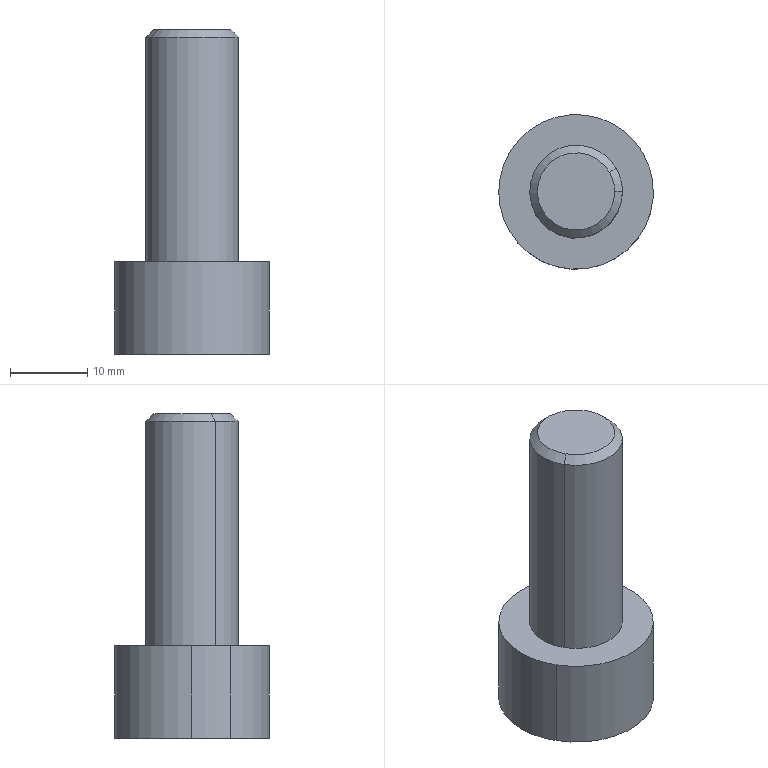Part | SolidWorks | features BaseBody 1 | 1 solid | 19 faces | box 20 x 20 x 42 mm | volume 6635 mm3 | plane 10 | cylinder 6 | cone 3 | commonest cylinder face diameters 12 x3 20 x3
STEP:
#1=CARTESIAN_POINT('',(127.379,873.749,686.107));
#2=VERTEX_POINT('',#1);
#3=CARTESIAN_POINT('',(128.245,874.249,685.107));
#4=VERTEX_POINT('',#3);
#5=CARTESIAN_POINT('',(127.379,873.749,686.107));
#6=DIRECTION('',(0.6124,0.3536,-0.7071));
#7=VECTOR('',#6,1000.);
#8=LINE('',#5,#7);
#9=EDGE_CURVE('',#2,#4,#8,.T.);
#10=ORIENTED_EDGE('',*,*,#9,.T.);
#11=CARTESIAN_POINT('',(117.853,868.249,685.107));
#12=VERTEX_POINT('',#11);
#13=CARTESIAN_POINT('',(123.049,871.249,685.107));
#14=DIRECTION('',(0.,0.,1.));
#15=DIRECTION('',(0.866,0.5,0.));
#16=AXIS2_PLACEMENT_3D('',#13,#14,#15);
#17=CIRCLE('',#16,6.);
#18=EDGE_CURVE('',#4,#12,#17,.T.);
#19=ORIENTED_EDGE('',*,*,#18,.T.);
#20=CARTESIAN_POINT('',(118.719,868.749,686.107));
#21=VERTEX_POINT('',#20);
#22=CARTESIAN_POINT('',(118.719,868.749,686.107));
#23=DIRECTION('',(-0.6124,-0.3536,-0.7071));
#24=VECTOR('',#23,1000.);
#25=LINE('',#22,#24);
#26=EDGE_CURVE('',#21,#12,#25,.T.);
#27=ORIENTED_EDGE('',*,*,#26,.F.);
#28=CARTESIAN_POINT('',(123.049,871.249,686.107));
#29=DIRECTION('',(0.,0.,-1.));
#30=DIRECTION('',(0.866,0.5,0.));
#31=AXIS2_PLACEMENT_3D('',#28,#29,#30);
#32=CIRCLE('',#31,5.);
#33=EDGE_CURVE('',#21,#2,#32,.T.);
#34=ORIENTED_EDGE('',*,*,#33,.T.);
#35=EDGE_LOOP('',(#10,#19,#27,#34));
#36=FACE_OUTER_BOUND('',#35,.T.);
#37=CARTESIAN_POINT('',(123.049,871.249,686.107));
#38=DIRECTION('',(0.,0.,-1.));
#39=DIRECTION('',(1.,0.,0.));
#40=AXIS2_PLACEMENT_3D('',#37,#38,#39);
#41=CONICAL_SURFACE('',#40,5.,0.7854);
#42=ADVANCED_FACE('',(#36),#41,.T.);
#43=ORIENTED_EDGE('',*,*,#33,.F.);
#44=CARTESIAN_POINT('',(128.049,871.249,686.107));
#45=VERTEX_POINT('',#44);
#46=CARTESIAN_POINT('',(123.049,871.249,686.107));
#47=DIRECTION('',(0.,0.,-1.));
#48=DIRECTION('',(0.866,0.5,0.));
#49=AXIS2_PLACEMENT_3D('',#46,#47,#48);
#50=CIRCLE('',#49,5.);
#51=EDGE_CURVE('',#45,#21,#50,.T.);
#52=ORIENTED_EDGE('',*,*,#51,.F.);
#53=CARTESIAN_POINT('',(123.049,871.249,686.107));
#54=DIRECTION('',(0.,0.,-1.));
#55=DIRECTION('',(0.866,0.5,0.));
#56=AXIS2_PLACEMENT_3D('',#53,#54,#55);
#57=CIRCLE('',#56,5.);
#58=EDGE_CURVE('',#2,#45,#57,.T.);
#59=ORIENTED_EDGE('',*,*,#58,.F.);
#60=EDGE_LOOP('',(#43,#52,#59));
#61=FACE_OUTER_BOUND('',#60,.T.);
#62=CARTESIAN_POINT('',(123.049,871.249,686.107));
#63=DIRECTION('',(0.,0.,1.));
#64=DIRECTION('',(1.,0.,0.));
#65=AXIS2_PLACEMENT_3D('',#62,#63,#64);
#66=PLANE('',#65);
#67=ADVANCED_FACE('',(#61),#66,.T.);
#68=CARTESIAN_POINT('',(128.245,874.249,656.107));
#69=VERTEX_POINT('',#68);
#70=CARTESIAN_POINT('',(128.245,874.249,686.107));
#71=DIRECTION('',(0.,0.,-1.));
#72=VECTOR('',#71,1000.);
#73=LINE('',#70,#72);
#74=EDGE_CURVE('',#4,#69,#73,.T.);
#75=ORIENTED_EDGE('',*,*,#74,.T.);
#76=CARTESIAN_POINT('',(117.853,868.249,656.107));
#77=VERTEX_POINT('',#76);
#78=CARTESIAN_POINT('',(123.049,871.249,656.107));
#79=DIRECTION('',(0.,0.,-1.));
#80=DIRECTION('',(-0.866,-0.5,0.));
#81=AXIS2_PLACEMENT_3D('',#78,#79,#80);
#82=CIRCLE('',#81,6.);
#83=EDGE_CURVE('',#77,#69,#82,.T.);
#84=ORIENTED_EDGE('',*,*,#83,.F.);
#85=CARTESIAN_POINT('',(117.853,868.249,686.107));
#86=DIRECTION('',(0.,0.,-1.));
#87=VECTOR('',#86,1000.);
#88=LINE('',#85,#87);
#89=EDGE_CURVE('',#12,#77,#88,.T.);
#90=ORIENTED_EDGE('',*,*,#89,.F.);
#91=ORIENTED_EDGE('',*,*,#18,.F.);
#92=EDGE_LOOP('',(#75,#84,#90,#91));
#93=FACE_OUTER_BOUND('',#92,.T.);
#94=CARTESIAN_POINT('',(123.049,871.249,686.107));
#95=DIRECTION('',(0.,0.,-1.));
#96=DIRECTION('',(1.,0.,0.));
#97=AXIS2_PLACEMENT_3D('',#94,#95,#96);
#98=CYLINDRICAL_SURFACE('',#97,6.);
#99=ADVANCED_FACE('',(#93),#98,.T.);
#100=CARTESIAN_POINT('',(121.262,876.683,650.107));
#101=VERTEX_POINT('',#100);
#102=CARTESIAN_POINT('',(117.449,872.418,650.107));
#103=VERTEX_POINT('',#102);
#104=CARTESIAN_POINT('',(121.262,876.683,650.107));
#105=DIRECTION('',(-0.6665,-0.7455,0.));
#106=VECTOR('',#105,1000.);
#107=LINE('',#104,#106);
#108=EDGE_CURVE('',#101,#103,#107,.T.);
#109=ORIENTED_EDGE('',*,*,#108,.F.);
#110=CARTESIAN_POINT('',(126.861,875.513,650.107));
#111=VERTEX_POINT('',#110);
#112=CARTESIAN_POINT('',(126.861,875.513,650.107));
#113=DIRECTION('',(-0.9789,0.2044,0.));
#114=VECTOR('',#113,1000.);
#115=LINE('',#112,#114);
#116=EDGE_CURVE('',#111,#101,#115,.T.);
#117=ORIENTED_EDGE('',*,*,#116,.F.);
#118=CARTESIAN_POINT('',(128.648,870.08,650.107));
#119=VERTEX_POINT('',#118);
#120=CARTESIAN_POINT('',(128.648,870.08,650.107));
#121=DIRECTION('',(-0.3124,0.9499,0.));
#122=VECTOR('',#121,1000.);
#123=LINE('',#120,#122);
#124=EDGE_CURVE('',#119,#111,#123,.T.);
#125=ORIENTED_EDGE('',*,*,#124,.F.);
#126=CARTESIAN_POINT('',(124.836,865.815,650.107));
#127=VERTEX_POINT('',#126);
#128=CARTESIAN_POINT('',(124.836,865.815,650.107));
#129=DIRECTION('',(0.6665,0.7455,0.));
#130=VECTOR('',#129,1000.);
#131=LINE('',#128,#130);
#132=EDGE_CURVE('',#127,#119,#131,.T.);
#133=ORIENTED_EDGE('',*,*,#132,.F.);
#134=CARTESIAN_POINT('',(119.237,866.984,650.107));
#135=VERTEX_POINT('',#134);
#136=CARTESIAN_POINT('',(119.237,866.984,650.107));
#137=DIRECTION('',(0.9789,-0.2044,0.));
#138=VECTOR('',#137,1000.);
#139=LINE('',#136,#138);
#140=EDGE_CURVE('',#135,#127,#139,.T.);
#141=ORIENTED_EDGE('',*,*,#140,.F.);
#142=CARTESIAN_POINT('',(117.449,872.418,650.107));
#143=DIRECTION('',(0.3124,-0.9499,0.));
#144=VECTOR('',#143,1000.);
#145=LINE('',#142,#144);
#146=EDGE_CURVE('',#103,#135,#145,.T.);
#147=ORIENTED_EDGE('',*,*,#146,.F.);
#148=EDGE_LOOP('',(#109,#117,#125,#133,#141,#147));
#149=FACE_OUTER_BOUND('',#148,.T.);
#150=CARTESIAN_POINT('',(117.449,872.418,650.107));
#151=DIRECTION('',(0.,0.,-1.));
#152=DIRECTION('',(0.,-1.,0.));
#153=AXIS2_PLACEMENT_3D('',#150,#151,#152);
#154=PLANE('',#153);
#155=ADVANCED_FACE('',(#149),#154,.T.);
#156=CARTESIAN_POINT('',(117.449,872.418,644.107));
#157=VERTEX_POINT('',#156);
#158=CARTESIAN_POINT('',(119.237,866.984,644.107));
#159=VERTEX_POINT('',#158);
#160=CARTESIAN_POINT('',(117.449,872.418,644.107));
#161=DIRECTION('',(0.3124,-0.9499,0.));
#162=VECTOR('',#161,1000.);
#163=LINE('',#160,#162);
#164=EDGE_CURVE('',#157,#159,#163,.T.);
#165=ORIENTED_EDGE('',*,*,#164,.F.);
#166=CARTESIAN_POINT('',(117.449,872.418,650.107));
#167=DIRECTION('',(0.,0.,-1.));
#168=VECTOR('',#167,1000.);
#169=LINE('',#166,#168);
#170=EDGE_CURVE('',#103,#157,#169,.T.);
#171=ORIENTED_EDGE('',*,*,#170,.F.);
#172=ORIENTED_EDGE('',*,*,#146,.T.);
#173=CARTESIAN_POINT('',(119.237,866.984,650.107));
#174=DIRECTION('',(0.,0.,-1.));
#175=VECTOR('',#174,1000.);
#176=LINE('',#173,#175);
#177=EDGE_CURVE('',#135,#159,#176,.T.);
#178=ORIENTED_EDGE('',*,*,#177,.T.);
#179=EDGE_LOOP('',(#165,#171,#172,#178));
#180=FACE_OUTER_BOUND('',#179,.T.);
#181=CARTESIAN_POINT('',(117.449,872.418,650.107));
#182=DIRECTION('',(-0.9499,-0.3124,0.));
#183=DIRECTION('',(-0.3124,0.9499,0.));
#184=AXIS2_PLACEMENT_3D('',#181,#182,#183);
#185=PLANE('',#184);
#186=ADVANCED_FACE('',(#180),#185,.F.);
#187=CARTESIAN_POINT('',(124.836,865.815,644.107));
#188=VERTEX_POINT('',#187);
#189=CARTESIAN_POINT('',(119.237,866.984,644.107));
#190=DIRECTION('',(0.9789,-0.2044,0.));
#191=VECTOR('',#190,1000.);
#192=LINE('',#189,#191);
#193=EDGE_CURVE('',#159,#188,#192,.T.);
#194=ORIENTED_EDGE('',*,*,#193,.F.);
#195=ORIENTED_EDGE('',*,*,#177,.F.);
#196=ORIENTED_EDGE('',*,*,#140,.T.);
#197=CARTESIAN_POINT('',(124.836,865.815,650.107));
#198=DIRECTION('',(0.,0.,-1.));
#199=VECTOR('',#198,1000.);
#200=LINE('',#197,#199);
#201=EDGE_CURVE('',#127,#188,#200,.T.);
#202=ORIENTED_EDGE('',*,*,#201,.T.);
#203=EDGE_LOOP('',(#194,#195,#196,#202));
#204=FACE_OUTER_BOUND('',#203,.T.);
#205=CARTESIAN_POINT('',(119.237,866.984,650.107));
#206=DIRECTION('',(-0.2044,-0.9789,0.));
#207=DIRECTION('',(-0.9789,0.2044,0.));
#208=AXIS2_PLACEMENT_3D('',#205,#206,#207);
#209=PLANE('',#208);
#210=ADVANCED_FACE('',(#204),#209,.F.);
#211=CARTESIAN_POINT('',(128.648,870.08,644.107));
#212=VERTEX_POINT('',#211);
#213=CARTESIAN_POINT('',(124.836,865.815,644.107));
#214=DIRECTION('',(0.6665,0.7455,0.));
#215=VECTOR('',#214,1000.);
#216=LINE('',#213,#215);
#217=EDGE_CURVE('',#188,#212,#216,.T.);
#218=ORIENTED_EDGE('',*,*,#217,.F.);
#219=ORIENTED_EDGE('',*,*,#201,.F.);
#220=ORIENTED_EDGE('',*,*,#132,.T.);
#221=CARTESIAN_POINT('',(128.648,870.08,650.107));
#222=DIRECTION('',(0.,0.,-1.));
#223=VECTOR('',#222,1000.);
#224=LINE('',#221,#223);
#225=EDGE_CURVE('',#119,#212,#224,.T.);
#226=ORIENTED_EDGE('',*,*,#225,.T.);
#227=EDGE_LOOP('',(#218,#219,#220,#226));
#228=FACE_OUTER_BOUND('',#227,.T.);
#229=CARTESIAN_POINT('',(124.836,865.815,650.107));
#230=DIRECTION('',(0.7455,-0.6665,0.));
#231=DIRECTION('',(0.,0.,-1.));
#232=AXIS2_PLACEMENT_3D('',#229,#230,#231);
#233=PLANE('',#232);
#234=ADVANCED_FACE('',(#228),#233,.F.);
#235=CARTESIAN_POINT('',(126.861,875.513,644.107));
#236=VERTEX_POINT('',#235);
#237=CARTESIAN_POINT('',(128.648,870.08,644.107));
#238=DIRECTION('',(-0.3124,0.9499,0.));
#239=VECTOR('',#238,1000.);
#240=LINE('',#237,#239);
#241=EDGE_CURVE('',#212,#236,#240,.T.);
#242=ORIENTED_EDGE('',*,*,#241,.F.);
#243=ORIENTED_EDGE('',*,*,#225,.F.);
#244=ORIENTED_EDGE('',*,*,#124,.T.);
#245=CARTESIAN_POINT('',(126.861,875.513,650.107));
#246=DIRECTION('',(0.,0.,-1.));
#247=VECTOR('',#246,1000.);
#248=LINE('',#245,#247);
#249=EDGE_CURVE('',#111,#236,#248,.T.);
#250=ORIENTED_EDGE('',*,*,#249,.T.);
#251=EDGE_LOOP('',(#242,#243,#244,#250));
#252=FACE_OUTER_BOUND('',#251,.T.);
#253=CARTESIAN_POINT('',(128.648,870.08,650.107));
#254=DIRECTION('',(0.9499,0.3124,0.));
#255=DIRECTION('',(0.,0.,-1.));
#256=AXIS2_PLACEMENT_3D('',#253,#254,#255);
#257=PLANE('',#256);
#258=ADVANCED_FACE('',(#252),#257,.F.);
#259=CARTESIAN_POINT('',(121.262,876.683,644.107));
#260=VERTEX_POINT('',#259);
#261=CARTESIAN_POINT('',(126.861,875.513,644.107));
#262=DIRECTION('',(-0.9789,0.2044,0.));
#263=VECTOR('',#262,1000.);
#264=LINE('',#261,#263);
#265=EDGE_CURVE('',#236,#260,#264,.T.);
#266=ORIENTED_EDGE('',*,*,#265,.F.);
#267=ORIENTED_EDGE('',*,*,#249,.F.);
#268=ORIENTED_EDGE('',*,*,#116,.T.);
#269=CARTESIAN_POINT('',(121.262,876.683,650.107));
#270=DIRECTION('',(0.,0.,-1.));
#271=VECTOR('',#270,1000.);
#272=LINE('',#269,#271);
#273=EDGE_CURVE('',#101,#260,#272,.T.);
#274=ORIENTED_EDGE('',*,*,#273,.T.);
#275=EDGE_LOOP('',(#266,#267,#268,#274));
#276=FACE_OUTER_BOUND('',#275,.T.);
#277=CARTESIAN_POINT('',(126.861,875.513,650.107));
#278=DIRECTION('',(0.2044,0.9789,0.));
#279=DIRECTION('',(0.,0.,-1.));
#280=AXIS2_PLACEMENT_3D('',#277,#278,#279);
#281=PLANE('',#280);
#282=ADVANCED_FACE('',(#276),#281,.F.);
#283=CARTESIAN_POINT('',(121.262,876.683,644.107));
#284=DIRECTION('',(-0.6665,-0.7455,0.));
#285=VECTOR('',#284,1000.);
#286=LINE('',#283,#285);
#287=EDGE_CURVE('',#260,#157,#286,.T.);
#288=ORIENTED_EDGE('',*,*,#287,.F.);
#289=ORIENTED_EDGE('',*,*,#273,.F.);
#290=ORIENTED_EDGE('',*,*,#108,.T.);
#291=ORIENTED_EDGE('',*,*,#170,.T.);
#292=EDGE_LOOP('',(#288,#289,#290,#291));
#293=FACE_OUTER_BOUND('',#292,.T.);
#294=CARTESIAN_POINT('',(121.262,876.683,650.107));
#295=DIRECTION('',(-0.7455,0.6665,0.));
#296=DIRECTION('',(0.,0.,1.));
#297=AXIS2_PLACEMENT_3D('',#294,#295,#296);
#298=PLANE('',#297);
#299=ADVANCED_FACE('',(#293),#298,.F.);
#300=ORIENTED_EDGE('',*,*,#287,.T.);
#301=ORIENTED_EDGE('',*,*,#164,.T.);
#302=ORIENTED_EDGE('',*,*,#193,.T.);
#303=ORIENTED_EDGE('',*,*,#217,.T.);
#304=ORIENTED_EDGE('',*,*,#241,.T.);
#305=ORIENTED_EDGE('',*,*,#265,.T.);
#306=EDGE_LOOP('',(#300,#301,#302,#303,#304,#305));
#307=FACE_BOUND('',#306,.T.);
#308=CARTESIAN_POINT('',(131.709,876.249,644.107));
#309=VERTEX_POINT('',#308);
#310=CARTESIAN_POINT('',(113.049,871.249,644.107));
#311=VERTEX_POINT('',#310);
#312=CARTESIAN_POINT('',(123.049,871.249,644.107));
#313=DIRECTION('',(0.,0.,1.));
#314=DIRECTION('',(-0.866,-0.5,0.));
#315=AXIS2_PLACEMENT_3D('',#312,#313,#314);
#316=CIRCLE('',#315,10.);
#317=EDGE_CURVE('',#309,#311,#316,.T.);
#318=ORIENTED_EDGE('',*,*,#317,.F.);
#319=CARTESIAN_POINT('',(114.388,866.249,644.107));
#320=VERTEX_POINT('',#319);
#321=CARTESIAN_POINT('',(123.049,871.249,644.107));
#322=DIRECTION('',(0.,0.,1.));
#323=DIRECTION('',(-0.866,-0.5,0.));
#324=AXIS2_PLACEMENT_3D('',#321,#322,#323);
#325=CIRCLE('',#324,10.);
#326=EDGE_CURVE('',#320,#309,#325,.T.);
#327=ORIENTED_EDGE('',*,*,#326,.F.);
#328=CARTESIAN_POINT('',(123.049,871.249,644.107));
#329=DIRECTION('',(0.,0.,1.));
#330=DIRECTION('',(-0.866,-0.5,0.));
#331=AXIS2_PLACEMENT_3D('',#328,#329,#330);
#332=CIRCLE('',#331,10.);
#333=EDGE_CURVE('',#311,#320,#332,.T.);
#334=ORIENTED_EDGE('',*,*,#333,.F.);
#335=EDGE_LOOP('',(#318,#327,#334));
#336=FACE_OUTER_BOUND('',#335,.T.);
#337=CARTESIAN_POINT('',(123.049,871.249,644.107));
#338=DIRECTION('',(0.,0.,-1.));
#339=DIRECTION('',(0.,-1.,0.));
#340=AXIS2_PLACEMENT_3D('',#337,#338,#339);
#341=PLANE('',#340);
#342=ADVANCED_FACE('',(#307,#336),#341,.T.);
#343=CARTESIAN_POINT('',(113.049,871.249,656.107));
#344=VERTEX_POINT('',#343);
#345=CARTESIAN_POINT('',(113.049,871.249,644.107));
#346=DIRECTION('',(0.,0.,1.));
#347=VECTOR('',#346,1000.);
#348=LINE('',#345,#347);
#349=EDGE_CURVE('',#311,#344,#348,.T.);
#350=ORIENTED_EDGE('',*,*,#349,.F.);
#351=ORIENTED_EDGE('',*,*,#333,.T.);
#352=CARTESIAN_POINT('',(114.388,866.249,656.107));
#353=VERTEX_POINT('',#352);
#354=CARTESIAN_POINT('',(114.388,866.249,644.107));
#355=DIRECTION('',(0.,0.,1.));
#356=VECTOR('',#355,1000.);
#357=LINE('',#354,#356);
#358=EDGE_CURVE('',#320,#353,#357,.T.);
#359=ORIENTED_EDGE('',*,*,#358,.T.);
#360=CARTESIAN_POINT('',(123.049,871.249,656.107));
#361=DIRECTION('',(0.,0.,1.));
#362=DIRECTION('',(-0.866,-0.5,0.));
#363=AXIS2_PLACEMENT_3D('',#360,#361,#362);
#364=CIRCLE('',#363,10.);
#365=EDGE_CURVE('',#344,#353,#364,.T.);
#366=ORIENTED_EDGE('',*,*,#365,.F.);
#367=EDGE_LOOP('',(#350,#351,#359,#366));
#368=FACE_OUTER_BOUND('',#367,.T.);
#369=CARTESIAN_POINT('',(123.049,871.249,644.107));
#370=DIRECTION('',(0.,0.,1.));
#371=DIRECTION('',(-1.,0.,0.));
#372=AXIS2_PLACEMENT_3D('',#369,#370,#371);
#373=CYLINDRICAL_SURFACE('',#372,10.);
#374=ADVANCED_FACE('',(#368),#373,.T.);
#375=ORIENTED_EDGE('',*,*,#83,.T.);
#376=CARTESIAN_POINT('',(129.049,871.249,656.107));
#377=VERTEX_POINT('',#376);
#378=CARTESIAN_POINT('',(123.049,871.249,656.107));
#379=DIRECTION('',(0.,0.,-1.));
#380=DIRECTION('',(-0.866,-0.5,0.));
#381=AXIS2_PLACEMENT_3D('',#378,#379,#380);
#382=CIRCLE('',#381,6.);
#383=EDGE_CURVE('',#69,#377,#382,.T.);
#384=ORIENTED_EDGE('',*,*,#383,.T.);
#385=CARTESIAN_POINT('',(123.049,871.249,656.107));
#386=DIRECTION('',(0.,0.,-1.));
#387=DIRECTION('',(-0.866,-0.5,0.));
#388=AXIS2_PLACEMENT_3D('',#385,#386,#387);
#389=CIRCLE('',#388,6.);
#390=EDGE_CURVE('',#377,#77,#389,.T.);
#391=ORIENTED_EDGE('',*,*,#390,.T.);
#392=EDGE_LOOP('',(#375,#384,#391));
#393=FACE_BOUND('',#392,.T.);
#394=CARTESIAN_POINT('',(131.709,876.249,656.107));
#395=VERTEX_POINT('',#394);
#396=CARTESIAN_POINT('',(123.049,871.249,656.107));
#397=DIRECTION('',(0.,0.,1.));
#398=DIRECTION('',(-0.866,-0.5,0.));
#399=AXIS2_PLACEMENT_3D('',#396,#397,#398);
#400=CIRCLE('',#399,10.);
#401=EDGE_CURVE('',#395,#344,#400,.T.);
#402=ORIENTED_EDGE('',*,*,#401,.T.);
#403=ORIENTED_EDGE('',*,*,#365,.T.);
#404=CARTESIAN_POINT('',(123.049,871.249,656.107));
#405=DIRECTION('',(0.,0.,1.));
#406=DIRECTION('',(-0.866,-0.5,0.));
#407=AXIS2_PLACEMENT_3D('',#404,#405,#406);
#408=CIRCLE('',#407,10.);
#409=EDGE_CURVE('',#353,#395,#408,.T.);
#410=ORIENTED_EDGE('',*,*,#409,.T.);
#411=EDGE_LOOP('',(#402,#403,#410));
#412=FACE_OUTER_BOUND('',#411,.T.);
#413=CARTESIAN_POINT('',(123.049,871.249,656.107));
#414=DIRECTION('',(0.,0.,-1.));
#415=DIRECTION('',(0.,-1.,0.));
#416=AXIS2_PLACEMENT_3D('',#413,#414,#415);
#417=PLANE('',#416);
#418=ADVANCED_FACE('',(#393,#412),#417,.F.);
#419=ORIENTED_EDGE('',*,*,#326,.T.);
#420=CARTESIAN_POINT('',(131.709,876.249,644.107));
#421=DIRECTION('',(0.,0.,1.));
#422=VECTOR('',#421,1000.);
#423=LINE('',#420,#422);
#424=EDGE_CURVE('',#309,#395,#423,.T.);
#425=ORIENTED_EDGE('',*,*,#424,.T.);
#426=ORIENTED_EDGE('',*,*,#409,.F.);
#427=ORIENTED_EDGE('',*,*,#358,.F.);
#428=EDGE_LOOP('',(#419,#425,#426,#427));
#429=FACE_OUTER_BOUND('',#428,.T.);
#430=CARTESIAN_POINT('',(123.049,871.249,644.107));
#431=DIRECTION('',(0.,0.,1.));
#432=DIRECTION('',(-1.,0.,0.));
#433=AXIS2_PLACEMENT_3D('',#430,#431,#432);
#434=CYLINDRICAL_SURFACE('',#433,10.);
#435=ADVANCED_FACE('',(#429),#434,.T.);
#436=CARTESIAN_POINT('',(129.049,871.249,685.107));
#437=VERTEX_POINT('',#436);
#438=CARTESIAN_POINT('',(129.049,871.249,686.107));
#439=DIRECTION('',(0.,0.,-1.));
#440=VECTOR('',#439,1000.);
#441=LINE('',#438,#440);
#442=EDGE_CURVE('',#437,#377,#441,.T.);
#443=ORIENTED_EDGE('',*,*,#442,.F.);
#444=CARTESIAN_POINT('',(123.049,871.249,685.107));
#445=DIRECTION('',(0.,0.,1.));
#446=DIRECTION('',(0.866,0.5,0.));
#447=AXIS2_PLACEMENT_3D('',#444,#445,#446);
#448=CIRCLE('',#447,6.);
#449=EDGE_CURVE('',#12,#437,#448,.T.);
#450=ORIENTED_EDGE('',*,*,#449,.F.);
#451=ORIENTED_EDGE('',*,*,#89,.T.);
#452=ORIENTED_EDGE('',*,*,#390,.F.);
#453=EDGE_LOOP('',(#443,#450,#451,#452));
#454=FACE_OUTER_BOUND('',#453,.T.);
#455=CARTESIAN_POINT('',(123.049,871.249,686.107));
#456=DIRECTION('',(0.,0.,-1.));
#457=DIRECTION('',(1.,0.,0.));
#458=AXIS2_PLACEMENT_3D('',#455,#456,#457);
#459=CYLINDRICAL_SURFACE('',#458,6.);
#460=ADVANCED_FACE('',(#454),#459,.T.);
#461=CARTESIAN_POINT('',(128.049,871.249,686.107));
#462=DIRECTION('',(0.7071,0.,-0.7071));
#463=VECTOR('',#462,1000.);
#464=LINE('',#461,#463);
#465=EDGE_CURVE('',#45,#437,#464,.T.);
#466=ORIENTED_EDGE('',*,*,#465,.F.);
#467=ORIENTED_EDGE('',*,*,#51,.T.);
#468=ORIENTED_EDGE('',*,*,#26,.T.);
#469=ORIENTED_EDGE('',*,*,#449,.T.);
#470=EDGE_LOOP('',(#466,#467,#468,#469));
#471=FACE_OUTER_BOUND('',#470,.T.);
#472=CARTESIAN_POINT('',(123.049,871.249,686.107));
#473=DIRECTION('',(0.,0.,-1.));
#474=DIRECTION('',(1.,0.,0.));
#475=AXIS2_PLACEMENT_3D('',#472,#473,#474);
#476=CONICAL_SURFACE('',#475,5.,0.7854);
#477=ADVANCED_FACE('',(#471),#476,.T.);
#478=ORIENTED_EDGE('',*,*,#58,.T.);
#479=ORIENTED_EDGE('',*,*,#465,.T.);
#480=CARTESIAN_POINT('',(123.049,871.249,685.107));
#481=DIRECTION('',(0.,0.,1.));
#482=DIRECTION('',(0.866,0.5,0.));
#483=AXIS2_PLACEMENT_3D('',#480,#481,#482);
#484=CIRCLE('',#483,6.);
#485=EDGE_CURVE('',#437,#4,#484,.T.);
#486=ORIENTED_EDGE('',*,*,#485,.T.);
#487=ORIENTED_EDGE('',*,*,#9,.F.);
#488=EDGE_LOOP('',(#478,#479,#486,#487));
#489=FACE_OUTER_BOUND('',#488,.T.);
#490=CARTESIAN_POINT('',(123.049,871.249,686.107));
#491=DIRECTION('',(0.,0.,-1.));
#492=DIRECTION('',(1.,0.,0.));
#493=AXIS2_PLACEMENT_3D('',#490,#491,#492);
#494=CONICAL_SURFACE('',#493,5.,0.7854);
#495=ADVANCED_FACE('',(#489),#494,.T.);
#496=ORIENTED_EDGE('',*,*,#485,.F.);
#497=ORIENTED_EDGE('',*,*,#442,.T.);
#498=ORIENTED_EDGE('',*,*,#383,.F.);
#499=ORIENTED_EDGE('',*,*,#74,.F.);
#500=EDGE_LOOP('',(#496,#497,#498,#499));
#501=FACE_OUTER_BOUND('',#500,.T.);
#502=CARTESIAN_POINT('',(123.049,871.249,686.107));
#503=DIRECTION('',(0.,0.,-1.));
#504=DIRECTION('',(1.,0.,0.));
#505=AXIS2_PLACEMENT_3D('',#502,#503,#504);
#506=CYLINDRICAL_SURFACE('',#505,6.);
#507=ADVANCED_FACE('',(#501),#506,.T.);
#508=ORIENTED_EDGE('',*,*,#317,.T.);
#509=ORIENTED_EDGE('',*,*,#349,.T.);
#510=ORIENTED_EDGE('',*,*,#401,.F.);
#511=ORIENTED_EDGE('',*,*,#424,.F.);
#512=EDGE_LOOP('',(#508,#509,#510,#511));
#513=FACE_OUTER_BOUND('',#512,.T.);
#514=CARTESIAN_POINT('',(123.049,871.249,644.107));
#515=DIRECTION('',(0.,0.,1.));
#516=DIRECTION('',(-1.,0.,0.));
#517=AXIS2_PLACEMENT_3D('',#514,#515,#516);
#518=CYLINDRICAL_SURFACE('',#517,10.);
#519=ADVANCED_FACE('',(#513),#518,.T.);
#520=CLOSED_SHELL('',(#42,#67,#99,#155,#186,#210,#234,#258,#282,#299,#342,#374,#418,#435,#460,#477,#495,#507,#519));
#521=MANIFOLD_SOLID_BREP('',#520);
#522=CARTESIAN_POINT('',(0.,0.,0.));
#523=DIRECTION('',(0.,0.,1.));
#524=DIRECTION('',(1.,0.,0.));
#525=AXIS2_PLACEMENT_3D('',#522,#523,#524);
#526=(LENGTH_UNIT()NAMED_UNIT(*)SI_UNIT(.MILLI.,.METRE.));
#527=UNCERTAINTY_MEASURE_WITH_UNIT(LENGTH_MEASURE(0.00001),#526,'','');
#528=(NAMED_UNIT(*)PLANE_ANGLE_UNIT()SI_UNIT($,.RADIAN.));
#529=(NAMED_UNIT(*)SI_UNIT($,.STERADIAN.)SOLID_ANGLE_UNIT());
#530=(GEOMETRIC_REPRESENTATION_CONTEXT(3)GLOBAL_UNCERTAINTY_ASSIGNED_CONTEXT((#527))GLOBAL_UNIT_ASSIGNED_CONTEXT((#526,#528,#529))REPRESENTATION_CONTEXT('',''));
#531=ADVANCED_BREP_SHAPE_REPRESENTATION('',(#521,#525),#530);